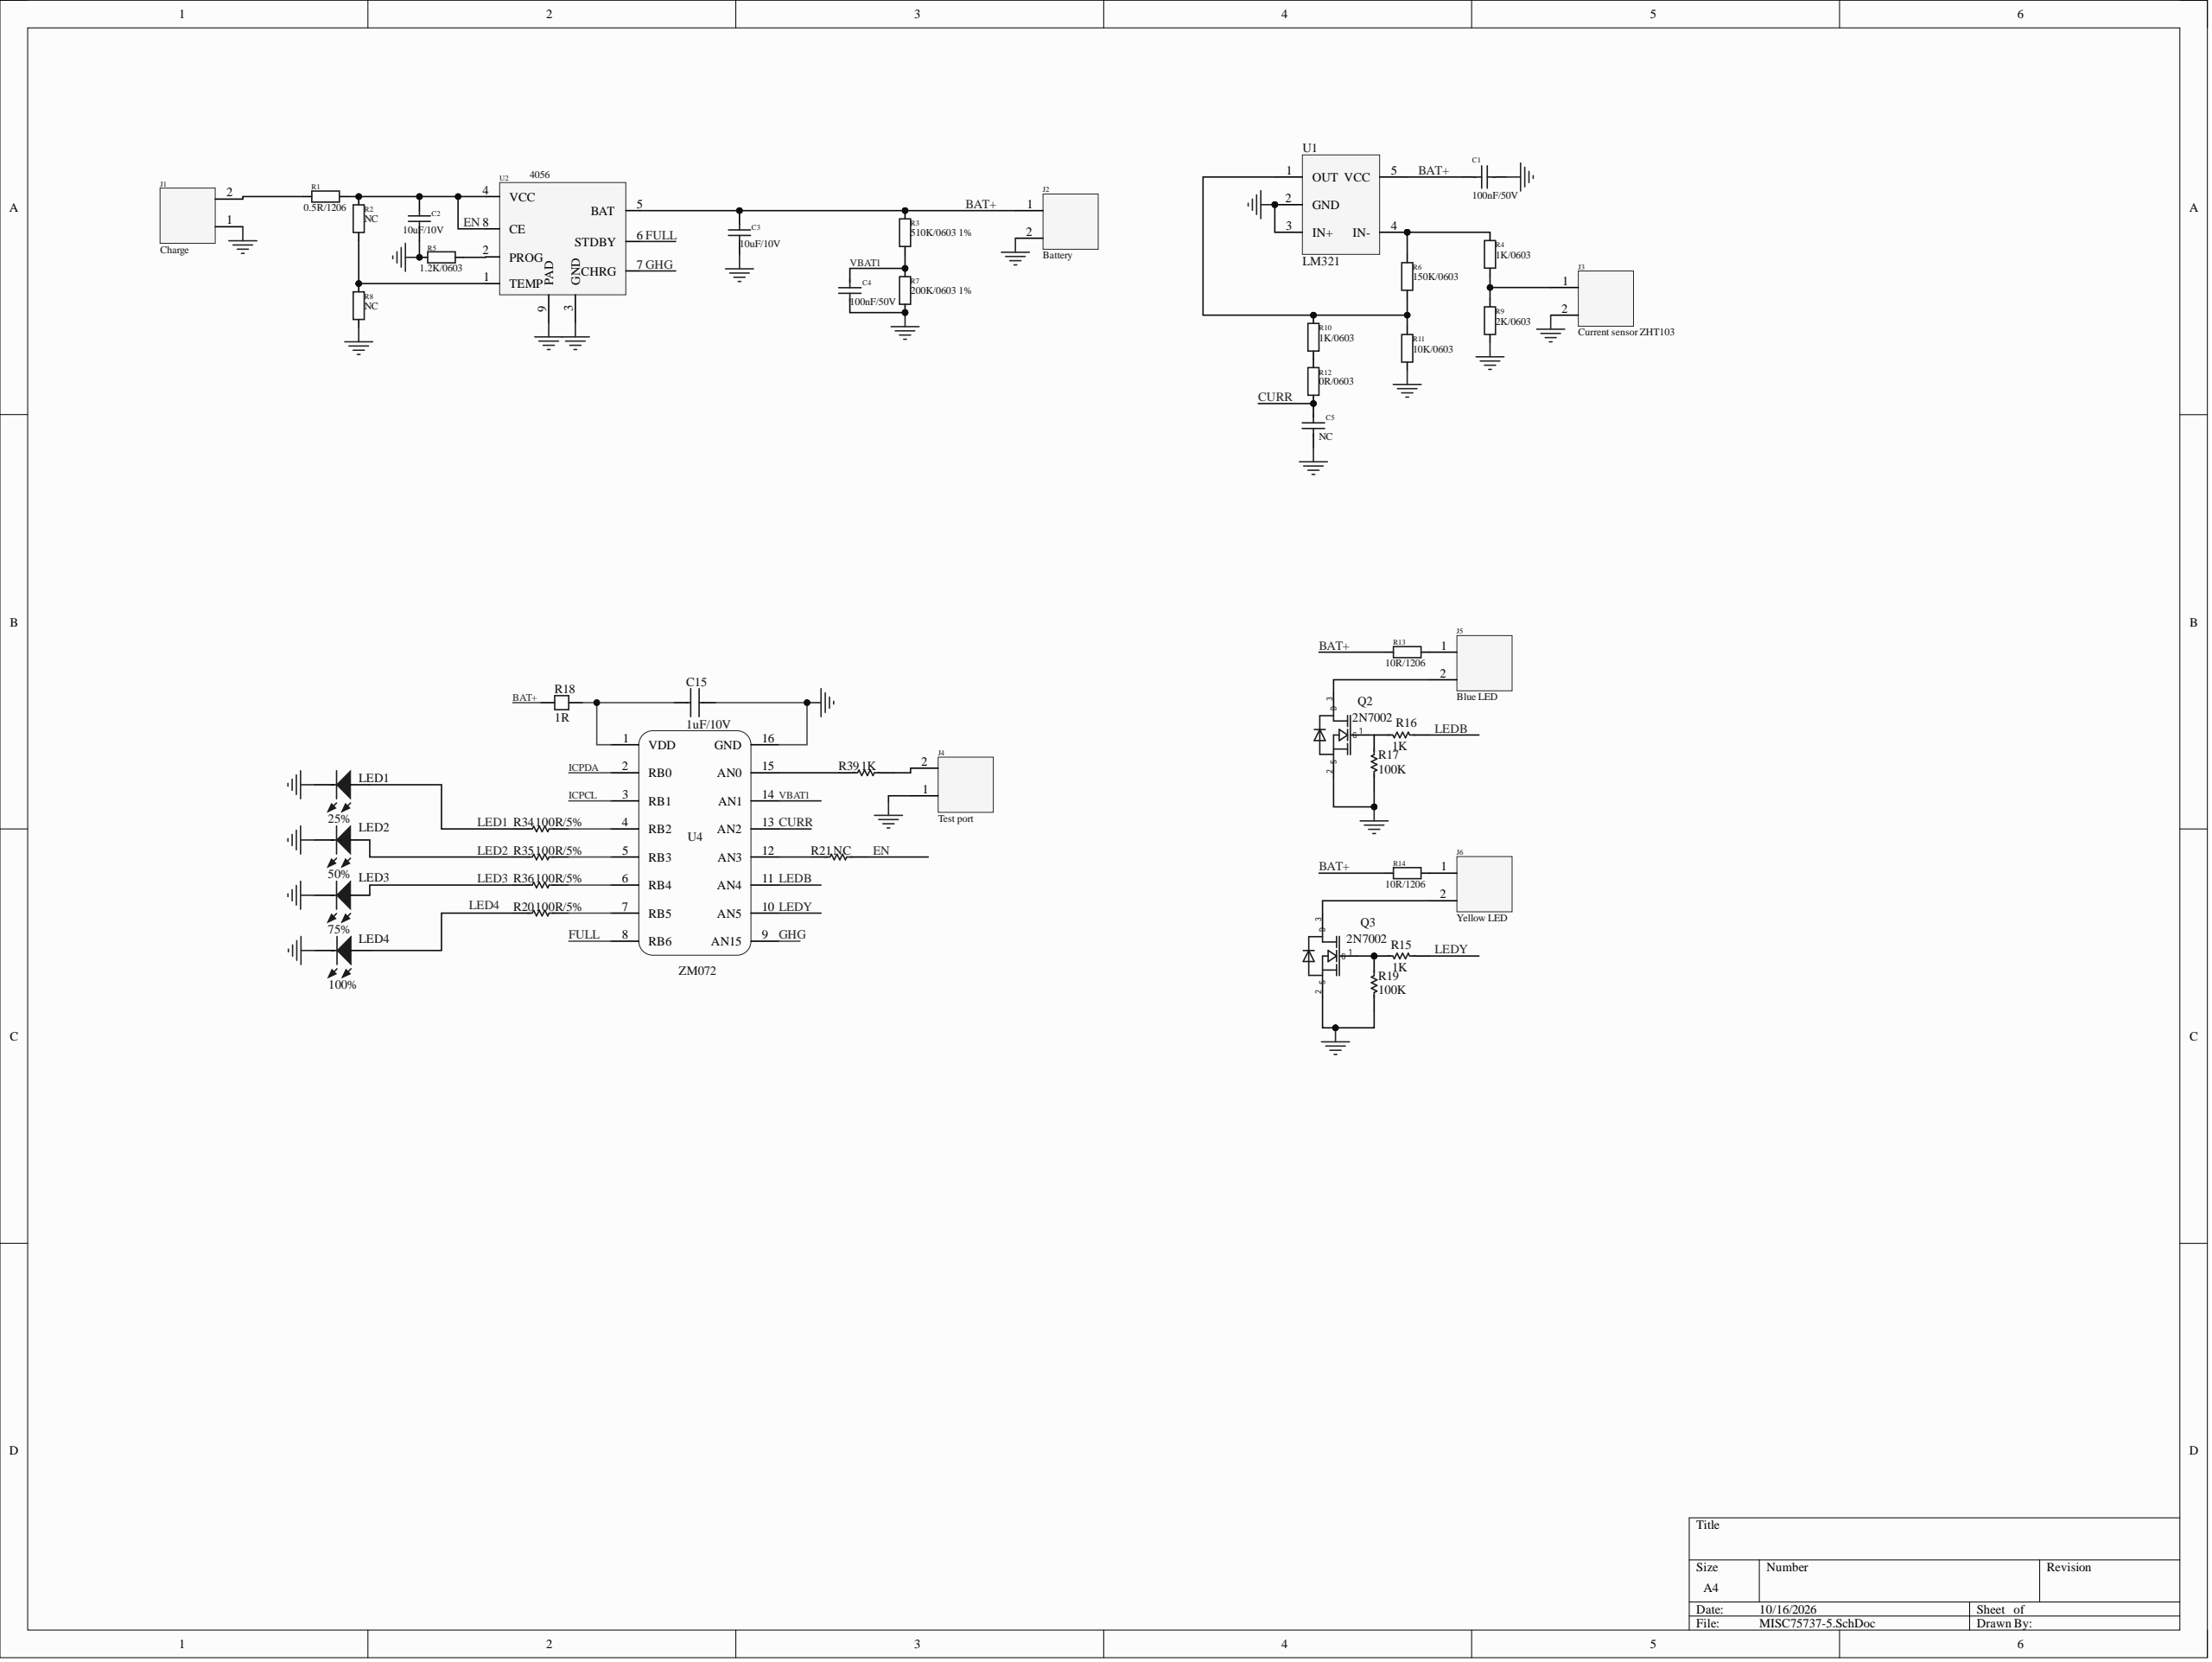Circuit board | Altium Designer | 46 parts | 34 nets
Bill of materials:
Comment,Description,Designator,Footprint,LibRef,Quantity
"100nF/50V","","C1, C4","C0603A","Cap0603","2"
"10uF/10V","SMD capacitor","C2, C3","C0805A","Cap0805","2"
"NC","","C5","C0603A","Cap0603","1"
"1uF/10V","","C15","C0603A","CH","1"
"Charge","DC socket right-angle 90° pitch 2.0","J1","HY2.0WT-2A/P 立贴带扣耐温260℃","2PIN","1"
"Battery","DC socket right-angle 90° pitch 2.0","J2","GH1.25-2PIN立贴带扣耐温260℃","2PIN","1"
"Current sensor ZHT103","DC socket right-angle 90° pitch 2.0","J3","IND-TH_L18.2-W10.2-P12.00-D0.9_ZHT103","2PIN","1"
"Test port","DC socket right-angle 90° pitch 2.0","J4","HY2.0WT-2A/P 立贴带扣耐温260℃","2PIN","1"
"Blue LED","DC socket right-angle 90° pitch 2.0","J5","GH1.25-2PIN立贴带扣耐温260℃","2PIN","1"
"Yellow LED","DC socket right-angle 90° pitch 2.0","J6","GH1.25-2PIN立贴带扣耐温260℃","2PIN","1"
"25%","SMD LED","LED1","LED0603A","LED 白发蓝","1"
"50%","SMD LED","LED2","LED0603A","LED 白发蓝","1"
"75%","SMD LED","LED3","LED0603A","LED 白发蓝","1"
"100%","SMD LED","LED4","LED0603A","LED 白发蓝","1"
"2N7002","SMD MOS","Q2, Q3","SOT23-3L","2N7002","2"
"0.5R/1206","SMD resistor","R1","R1206A","Res1206","1"
"NC","SMD resistor","R2, R8, R21","R0603A","Res0603","3"
"510K/0603 1%","SMD resistor","R3","R0603A","Res0603","1"
"1K/0603","SMD resistor","R4, R10","R0603A","Res0603","2"
"1.2K/0603","SMD resistor","R5","R0603A","Res0603","1"
"150K/0603","SMD resistor","R6","R0603A","Res0603","1"
"200K/0603 1%","SMD resistor","R7","R0603A","Res0603","1"
"2K/0603","SMD resistor","R9","R0603A","Res0603","1"
"10K/0603","SMD resistor","R11","R0603A","Res0603","1"
"0R/0603","SMD resistor","R12","R0603A","Res0603","1"
"10R/1206","SMD resistor","R13, R14","R1206A","Res1206","2"
"1K","SMD resistor","R15, R16, R39","R0603A","Res0603","3"
"100K","SMD resistor","R17, R19","R0603A","Res0603","2"
"1R","","R18","R0603A","RH1","1"
"100R/5%","SMD resistor","R20, R34, R35, R36","R0603A","Res0603","4"
"LM321","","U1","SOT23-5A","LM321","1"
"4056","Charger IC","U2","ESOP-8L","TP4056","1"
"ZM072","","U4","SOP16L","MCU-TSSOP-16","1"
Netlist (Protel format):
[
C1
C0603A
100nF/50V



]
[
C2
C0805A
10uF/10V



]
[
C3
C0805A
10uF/10V



]
[
C4
C0603A
100nF/50V



]
[
C5
C0603A
NC



]
[
C15
C0603A
1uF/10V



]
[
J1
HY2.0WT-2A/P 立贴带扣耐温260℃
Charge



]
[
J2
GH1.25-2PIN立贴带扣耐温260℃
Battery



]
[
J3
IND-TH_L18.2-W10.2-P12.00-D0.9_ZHT103
Current sensor ZHT103



]
[
J4
HY2.0WT-2A/P 立贴带扣耐温260℃
Test port



]
[
J5
GH1.25-2PIN立贴带扣耐温260℃
Blue LED



]
[
J6
GH1.25-2PIN立贴带扣耐温260℃
Yellow LED



]
[
LED1
LED0603A
25%



]
[
LED2
LED0603A
50%



]
[
LED3
LED0603A
75%



]
[
LED4
LED0603A
100%



]
[
Q2
SOT23-3L
2N7002



]
[
Q3
SOT23-3L
2N7002



]
[
R1
R1206A
0.5R/1206



]
[
R2
R0603A
NC



]
[
R3
R0603A
510K/0603 1%



]
[
R4
R0603A
1K/0603



]
[
R5
R0603A
1.2K/0603



]
[
R6
R0603A
150K/0603



]
[
R7
R0603A
200K/0603 1%



]
[
R8
R0603A
NC



]
[
R9
R0603A
2K/0603



]
[
R10
R0603A
1K/0603



]
[
R11
R0603A
10K/0603



]
[
R12
R0603A
0R/0603



]
[
R13
R1206A
10R/1206



]
[
R14
R1206A
10R/1206



]
[
R15
R0603A
1K



]
[
R16
R0603A
1K



]
[
R17
R0603A
100K



]
[
R18
R0603A
1R



]
[
R19
R0603A
100K



]
[
R20
R0603A
100R/5%



]
[
R21
R0603A
NC



]
[
R34
R0603A
100R/5%



]
[
R35
R0603A
100R/5%



]
[
R36
R0603A
100R/5%



]
[
R39
R0603A
1K



]
[
U1
SOT23-5A
LM321



]
[
U2
ESOP-8L
4056



]
[
U4
SOP16L
ZM072



]
(
VBAT1
C4-2
R3-1
R7-2
U4-14
)
(
NetR39_1
R39-1
U4-15
)
(
NetR36_2
R36-2
U4-6
)
(
NetR35_2
R35-2
U4-5
)
(
NetR34_2
R34-2
U4-4
)
(
NetR21_1
R21-1
U4-12
)
(
NetR20_2
R20-2
U4-7
)
(
NetR10_2
R10-2
R12-1
)
(
NetR6_2
R6-2
R10-1
R11-1
U1-1
)
(
NetR5_2
R5-2
U2-2
)
(
NetR4_1
R4-1
R6-1
U1-4
)
(
NetR2_1
R2-1
R8-2
U2-1
)
(
NetQ3_1
Q3-1
R15-1
R19-2
)
(
NetQ2_1
Q2-1
R16-1
R17-2
)
(
NetLED4_1
LED4-1
R20-1
)
(
NetJ6_2
J6-2
Q3-3
)
(
NetJ6_1
J6-1
R14-2
)
(
NetJ5_2
J5-2
Q2-3
)
(
NetJ5_1
J5-1
R13-2
)
(
NetJ4_2
J4-2
R39-2
)
(
NetJ3_1
J3-1
R4-2
R9-1
)
(
NetJ1_2
J1-2
R1-1
)
(
NetC15_1
C15-1
R18-2
U4-1
)
(
LEDY
R15-2
U4-10
)
(
LEDB
R16-2
U4-11
)
(
LED3
LED3-1
R36-1
)
(
LED2
LED2-1
R35-1
)
(
LED1
LED1-1
R34-1
)
(
GND
C1-1
C2-1
C3-1
C4-1
C5-1
C15-2
J1-1
J2-2
J3-2
J4-1
LED1-2
LED2-2
LED3-2
LED4-2
Q2-2
Q3-2
R5-1
R7-1
R8-1
R9-2
R11-2
R17-1
R19-1
U1-2
U1-3
U2-3
U2-9
U4-16
)
(
GHG
U2-7
U4-9
)
(
FULL
U2-6
U4-8
)
(
EN
C2-2
R1-2
R2-2
R21-2
U2-4
U2-8
)
(
CURR
C5-2
R12-2
U4-13
)
(
BAT+
C1-2
C3-2
J2-1
R3-2
R13-1
R14-1
R18-1
U1-5
U2-5
)